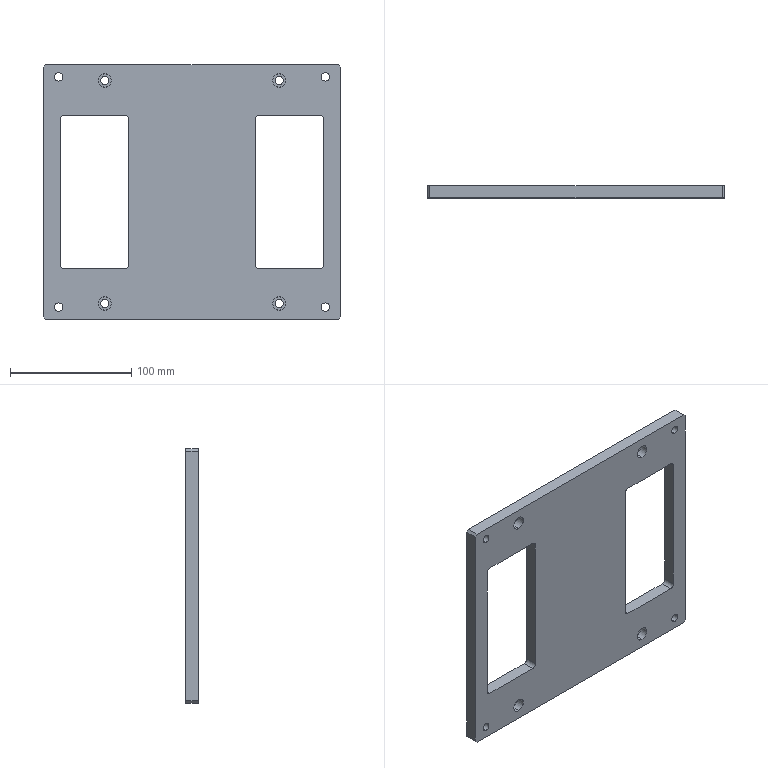Part | SolidWorks | features MirrorPattern 3, 3DProfileFeature 1, Chamfer 1, Cut 1, Extrusion 1, HoleWzd 1, ICE 1 | 1 solid | 62 faces | box 245 x 10 x 210 mm | volume 367454 mm3 | cylinder 32 | plane 22 | cone 8 | commonest cylinder face diameters 6.4 x8 6.6 x8 7 x8 11 x8